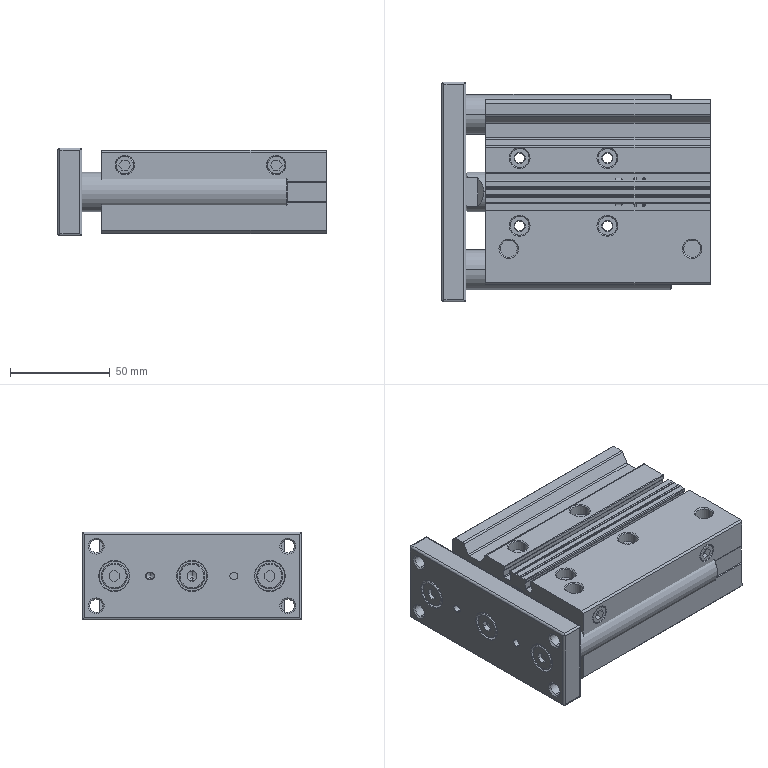Part | SolidWorks | 4 solids | 575 faces | box 134.5 x 110 x 44 mm | volume 443545 mm3 | cylinder 240 | plane 205 | cone 108 | spline 22 | commonest cylinder face diameters 0.4 x34 0.8 x28 2 x24 4 x18 4.917 x16 1.5 x11